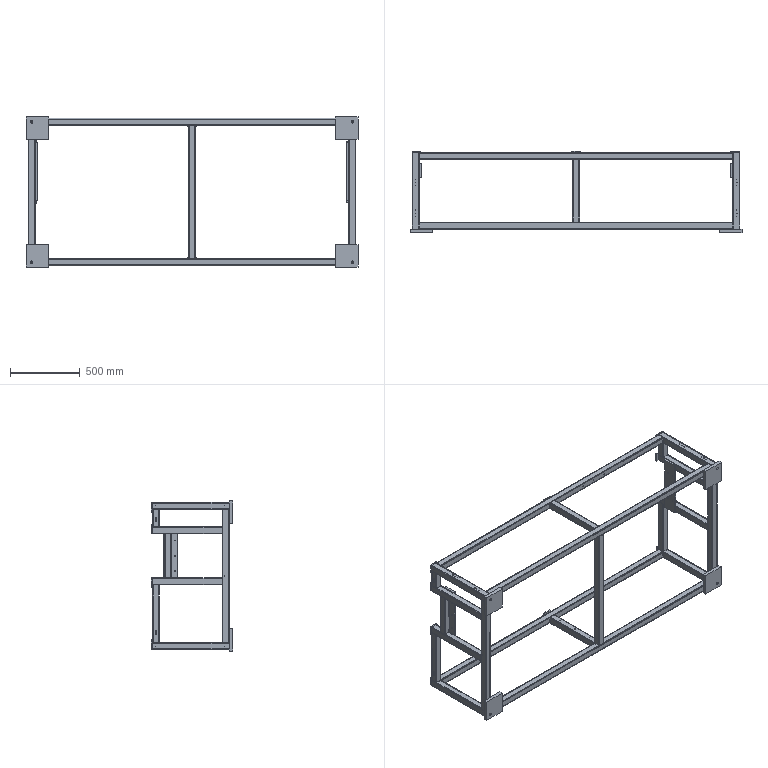Part | NX | features BREP 37 | 37 solids | 772 faces | box 2381 x 583 x 1076 mm | volume 12673960 mm3 | cylinder 445 | plane 327 | commonest cylinder face diameters 3.3 x140 10 x103 5 x92 6.8 x60 14 x36 17.5 x8